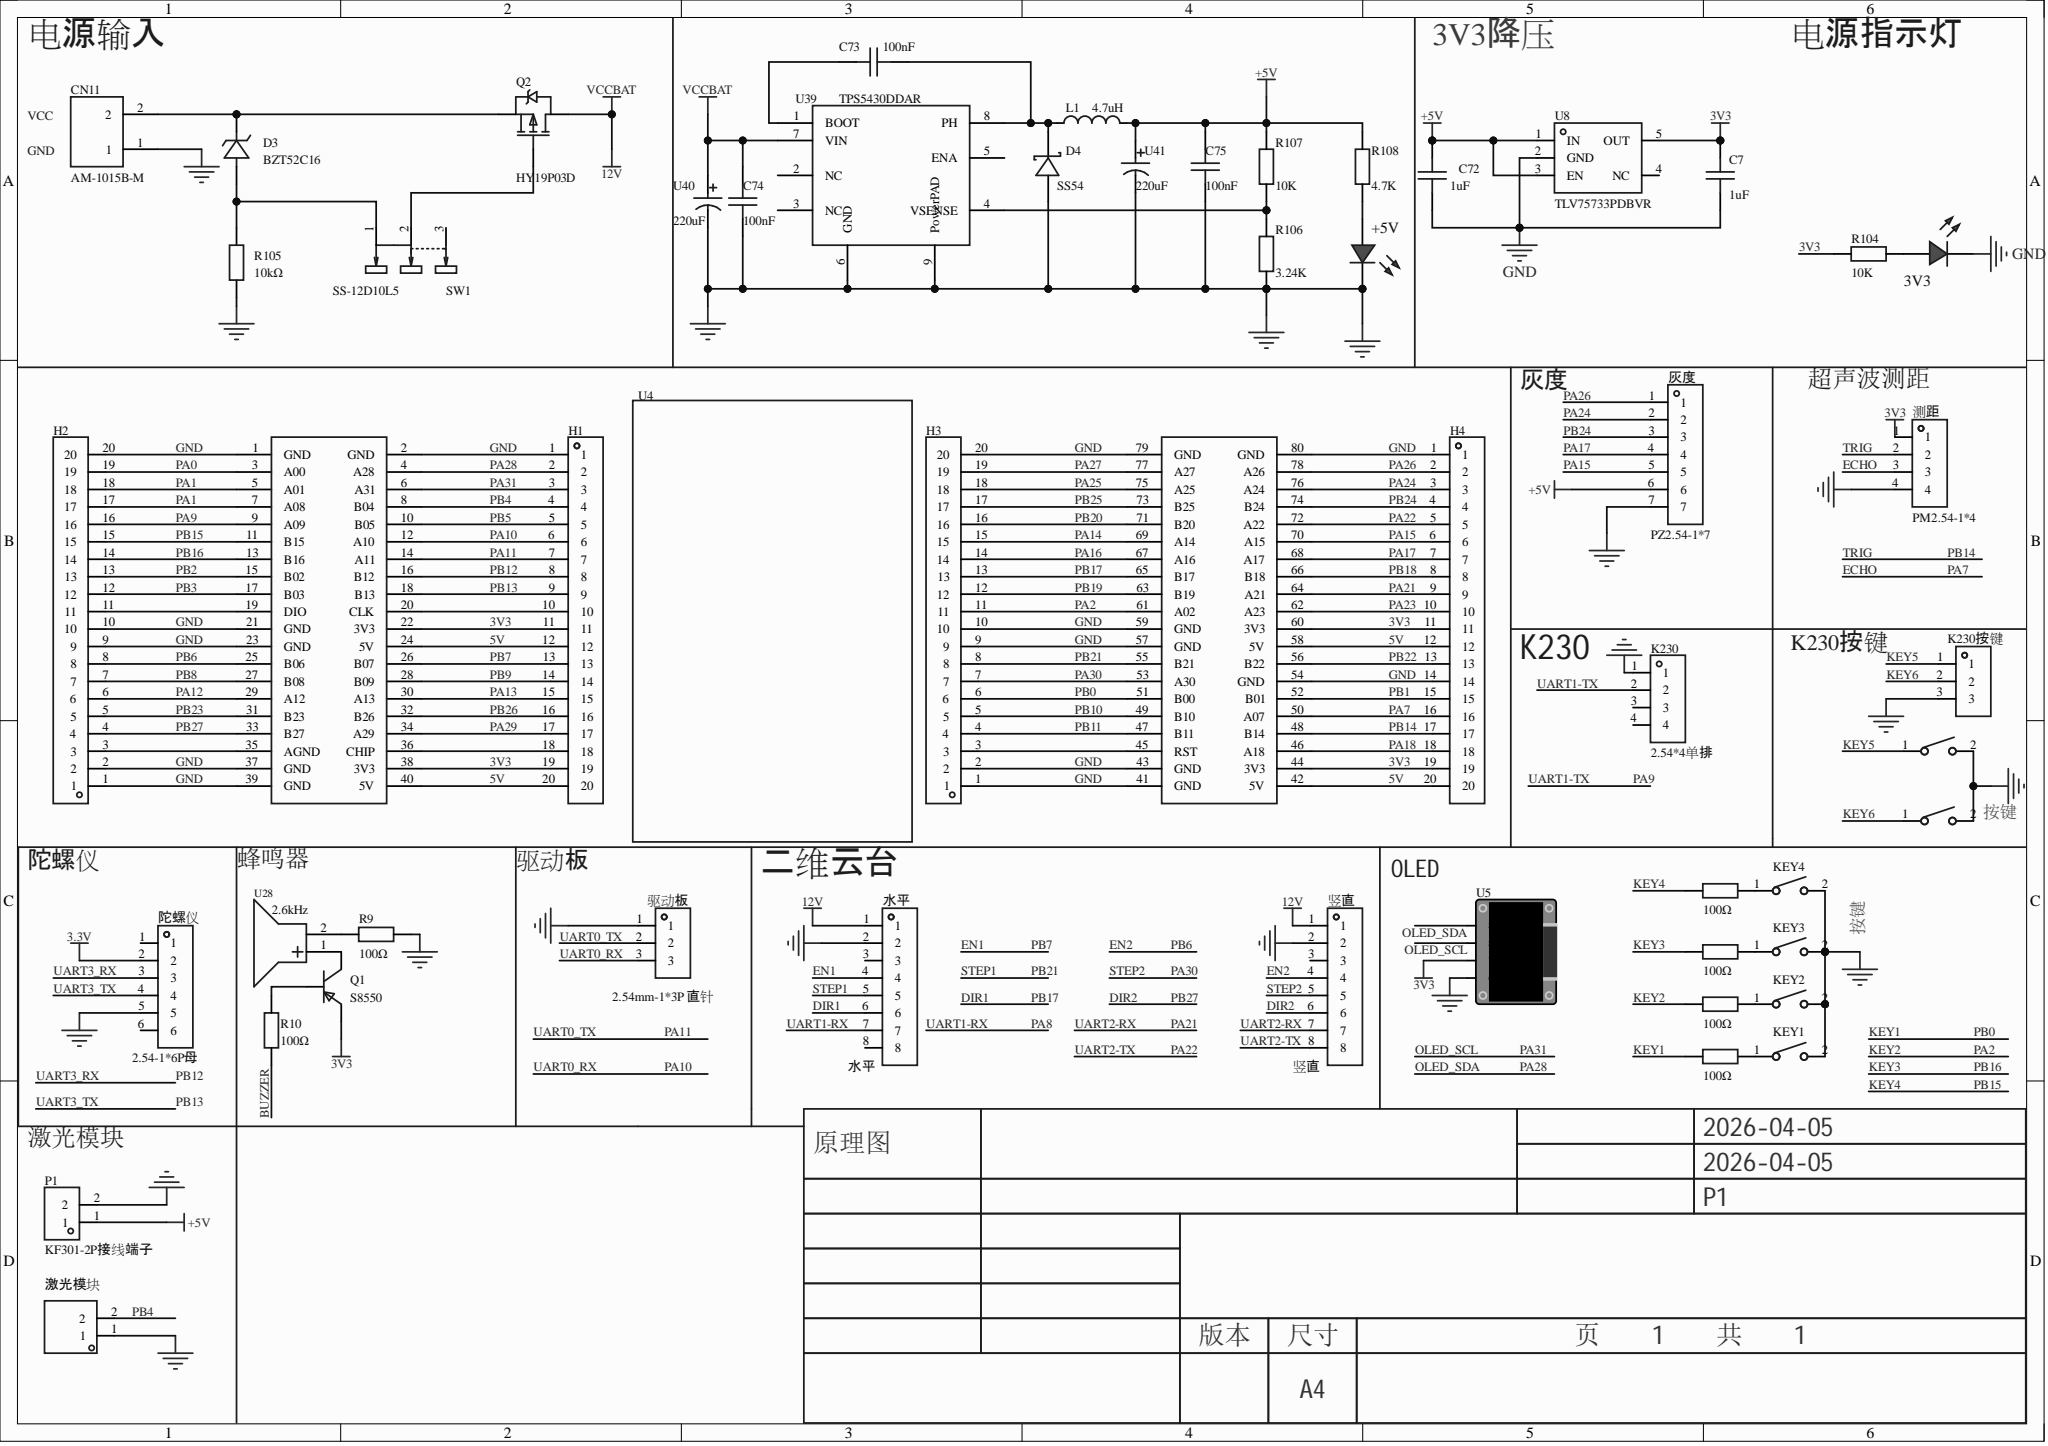Circuit board | Altium Designer | 52 parts | 80 nets
Bill of materials:
Comment,Description,Designator,Footprint,LibRef,Quantity
"","","+5V, 3V3","LED_0603","LED_0603-R","2"
"1uF","","C7, C72","C0603","CAP_0603","2"
"100nF","容值:100nF;精度:±10%;额定电压:50V;温度系数:X7R;","C73, C74, C75","C0805","CC0805KRX7R9BB104","3"
"AM-1015B-M","金属材质：铜镀金  绝缘材质：PA","CN11","CONN-TH_AM-1015B-M","AM-1015B-M","1"
"BZT52C16","二极管配置:独立式;稳压值(标称值):16V;稳压值(范围):15.3V~17.1V;耗散功率(Pd):500mW;","D3","SOD-123_L2.7-W1.6-LS3.7-RD","BZT52C16","1"
"SS54","二极管配置:独立式;正向压降(Vf):550mV@5A;直流反向耐压(Vr):40V;整流电流:5A;","D4","SMA_L4.4-W2.8-LS5.4-R-RD","SS54_C22452","1"
"","间距:2.54mm;总PIN位数:20;排数:1;插针结构:-;行距:-;安装类型:直插;圆针/方针:-;额定电流:-;额定电压:-;配合针长度:-;塑高:-;触头材质:黄铜;触头镀层:-;颜色:黑色;","H1, H2, H3, H4","HDR-TH_20P-P2.54-V-M-1","HDR-M_2.54_1x20P","4"
"2.54*4单排","","K230","HDR-TH_4P-P2.54-V-M-1","2.54*4单排","1"
"K230按键","","K230按键","HDR-TH_3P-P2.54-V-M","HDR-M_2.54_1x3P","1"
"轻触按键3*6*2.5","","K230按键1, K230按键2, KEY1, KEY2, KEY3, KEY4","SW-SMD_L6.0-W3.6-LS8.0","轻触按键3*6*2.5","6"
"4.7uH","电感值:4.7uH;精度:±20%;额定电流:5.5A;饱和电流(Isat):7A;","L1","IND-SMD_L7.3-W6.6","MCS0630-4R7MPY1","1"
"KF301-2P接线端子","","P1","CONN-TH_XY301V-A-5.0-2P","KF301-2P接线端子","1"
"S8550","晶体管类型:PNP;集电极电流(Ic):500mA;集射极击穿电压(Vceo):25V;功率(Pd):300mW;直流电流增益(hFE@Ic,Vce):120@50mA,1V;","Q1","SOT-23-3_L2.9-W1.6-P1.90-LS2.8-BR","S8550_C105432","1"
"HY19P03D","","Q2","TO-252-2_L6.6-W6.1-P4.57-LS9.9-TL-CW","HY19P03D","1"
"100Ω","","R9, R10, R109, R110, R111, R112","R0603","Res_0603, 0603WAF1000T5E","6"
"10K","","R104, R107","R0603","Res_0603","2"
"10kΩ","","R105","R0603","0603WAF1002T5E","1"
"3.24K","","R106","R0603","Res_0603","1"
"4.7K","","R108","R0603","Res_0603","1"
"SS-12D10L5","电路结构:单刀双掷;安装方式:直插;开关颜色:黑色;额定电流(DC):3A;额定电压(DC):125V;额定电流(AC):3A;额定电压(AC):125V;机械寿命:1万次;","SW1","SW-TH_SS-12D10L5","SS-12D10L5","1"
"","","U4","COMM-TH_LCKFB-TMX-MSPM0G3507","LCKFB-TMX-MSPM0G3507","1"
"","","U5","0.96OLED_4P","0.96OLED模块_4P","1"
"TLV75733PDBVR","输出类型:固定;最大输入电压:5.5V;输出电压:3.3V;输出电流:1A;电源纹波抑制比(PSRR):52dB;输出极性:正极;","U8","SOT-23-5_L2.9-W1.6-P0.95-LS2.8-BL","TLV75733PDBVR","1"
"2.6kHz","频率:2.6kHz;声压(SPL):80dB@5V,10cm;","U28","BUZ-TH_BD12.0-P7.60-D0.6-FD","HYE1206-05ST","1"
"TPS5430DDAR","功能类型:降压型;输出类型:可调;输入电压:5.5V~36V;输出电压:1.221V~32.04V;输出电流(最大值):3A;","U39","ESOP-8_L4.9-W3.9-P1.27-LS6.0-TL-EP","TPS5430DDAR","1"
"220uF","","U40, U41","CAP-SMD_BD6.3-L6.6-W6.6-LS7.2-FD","220uF","2"
"","","","CONN-TH_8P-P2.50-XH2.54-8P","XH2.54-8P 直插","1"
"PM2.54-1*4","插孔结构:1x4P;间距:2.54mm;行距:2.54mm;圆孔/方孔:方孔;安装方式:直插;排数:单排;总孔位数:4P;额定电流:2.5A;插孔方向:顶部;塑高:8.5mm;工作温度:-40℃~+105℃;","测距","HDR-TH_4P-P2.54-V-F","PM2.54-1*4","1"
"","","激光模块","HDR-TH_2P-P2.54-V-M-1","HDR-M_2.54_1x2P","1"
"PZ2.54-1*7","插针结构:1x7P;间距:2.54mm;圆针/方针:方针;安装方式:直插;排数:单排;总PIN位数:7P;额定电流:2.5A;配合针长度:6mm;塑高:2.54mm;端接针长度:3mm;触头材质:黄铜;触头镀层:金;工作温度:-40℃~+105℃;","灰度","HDR-TH_7P-P2.54-V-M","PZ2.54-1*7","1"
"","","","CONN-TH_8P-P2.50-XH2.54-8P","XH2.54-8P 直插","1"
"2.54-1*6P母","插孔结构:1x6P;间距:2.54mm;行距:-;圆孔/方孔:方孔;安装方式:直插;排数:单排;总孔位数:6P;额定电流:3A;额定电压:-;插孔方向:顶部;塑高:-;触头材质:黄铜;触头镀层:-;工作温度:-40℃~+105℃;","陀螺仪","HDR-TH_6P-P2.54-V-F","2.54-1*6P母","1"
"2.54mm-1*3P 直针","","驱动板","HDR-TH_3P-P2.54-V-M-1","2.54mm-1*3P 直针","1"
Netlist (Protel format):
[
3V3
LED_0603




]
[
+5V
LED_0603




]
[
C7
C0603
1uF



]
[
C72
C0603
1uF



]
[
C73
C0805
100nF



]
[
C74
C0805
100nF



]
[
C75
C0805
100nF



]
[
CN11
CONN-TH_AM-1015B-M
AM-1015B-M



]
[
D3
SOD-123_L2.7-W1.6-LS3.7-RD
BZT52C16



]
[
D4
SMA_L4.4-W2.8-LS5.4-R-RD
SS54



]
[
H1
HDR-TH_20P-P2.54-V-M-1




]
[
H2
HDR-TH_20P-P2.54-V-M-1




]
[
H3
HDR-TH_20P-P2.54-V-M-1




]
[
H4
HDR-TH_20P-P2.54-V-M-1




]
[
K230
HDR-TH_4P-P2.54-V-M-1
2.54*4单排



]
[
K230按键
HDR-TH_3P-P2.54-V-M
K230按键



]
[
K230按键1
SW-SMD_L6.0-W3.6-LS8.0
轻触按键3*6*2.5



]
[
K230按键2
SW-SMD_L6.0-W3.6-LS8.0
轻触按键3*6*2.5



]
[
KEY1
SW-SMD_L6.0-W3.6-LS8.0
轻触按键3*6*2.5



]
[
KEY2
SW-SMD_L6.0-W3.6-LS8.0
轻触按键3*6*2.5



]
[
KEY3
SW-SMD_L6.0-W3.6-LS8.0
轻触按键3*6*2.5



]
[
KEY4
SW-SMD_L6.0-W3.6-LS8.0
轻触按键3*6*2.5



]
[
L1
IND-SMD_L7.3-W6.6
4.7uH



]
[
P1
CONN-TH_XY301V-A-5.0-2P
KF301-2P接线端子



]
[
Q1
SOT-23-3_L2.9-W1.6-P1.90-LS2.8-BR
S8550



]
[
Q2
TO-252-2_L6.6-W6.1-P4.57-LS9.9-TL-CW
HY19P03D



]
[
R9
R0603
100Ω



]
[
R10
R0603
100Ω



]
[
R104
R0603
10K



]
[
R105
R0603
10kΩ



]
[
R106
R0603
3.24K



]
[
R107
R0603
10K



]
[
R108
R0603
4.7K



]
[
R109
R0603
100Ω



]
[
R110
R0603
100Ω



]
[
R111
R0603
100Ω



]
[
R112
R0603
100Ω



]
[
SW1
SW-TH_SS-12D10L5
SS-12D10L5



]
[
U4
COMM-TH_LCKFB-TMX-MSPM0G3507




]
[
U5
0.96OLED_4P




]
[
U8
SOT-23-5_L2.9-W1.6-P0.95-LS2.8-BL
TLV75733PDBVR



]
[
U28
BUZ-TH_BD12.0-P7.60-D0.6-FD
2.6kHz



]
[
U39
ESOP-8_L4.9-W3.9-P1.27-LS6.0-TL-EP
TPS5430DDAR



]
[
U40
CAP-SMD_BD6.3-L6.6-W6.6-LS7.2-FD
220uF



]
[
U41
CAP-SMD_BD6.3-L6.6-W6.6-LS7.2-FD
220uF



]
[
水平
CONN-TH_8P-P2.50-XH2.54-8P
水平



]
[
测距
HDR-TH_4P-P2.54-V-F
PM2.54-1*4



]
[
激光模块
HDR-TH_2P-P2.54-V-M-1




]
[
灰度
HDR-TH_7P-P2.54-V-M
PZ2.54-1*7



]
[
竖直
CONN-TH_8P-P2.50-XH2.54-8P
竖直



]
[
陀螺仪
HDR-TH_6P-P2.54-V-F
2.54-1*6P母



]
[
驱动板
HDR-TH_3P-P2.54-V-M-1
2.54mm-1*3P 直针



]
(
PB26
H1-16
U4-32
)
(
PB25
H3-17
U4-73
)
(
PB24
H4-4
U4-74
灰度-3
)
(
PB23
H2-5
U4-31
)
(
PB22
H4-13
U4-56
)
(
PB21
H3-8
U4-55
水平-5
)
(
PB20
H3-16
U4-71
)
(
PB19
H3-12
U4-63
)
(
PB18
H4-8
U4-66
)
(
PB14
H4-17
U4-48
测距-2
)
(
PB13
H1-9
U4-18
陀螺仪-4
)
(
PB12
H1-8
U4-16
陀螺仪-3
)
(
PB11
H3-4
U4-47
)
(
PB10
H3-5
U4-49
)
(
PB9
H1-14
U4-28
)
(
PB8
H2-7
U4-27
)
(
PB5
H1-5
U4-10
)
(
PB4
H1-4
U4-8
激光模块-2
)
(
PB3
H2-12
U4-17
)
(
PB2
H2-13
U4-15
)
(
PB1
H4-15
U4-52
)
(
PA30
H3-7
U4-53
竖直-5
)
(
PA29
H1-17
U4-34
)
(
PA27
H3-19
U4-77
)
(
PA26
H4-2
U4-78
灰度-1
)
(
PA25
H3-18
U4-75
)
(
PA24
H4-3
U4-76
灰度-2
)
(
PA23
H4-10
U4-62
)
(
PA22
H4-5
U4-72
竖直-8
)
(
PA21
H4-9
U4-64
竖直-7
)
(
PA18
H4-18
U4-46
)
(
PA17
H4-7
U4-68
灰度-4
)
(
PA16
H3-14
U4-67
)
(
PA15
H4-6
U4-70
灰度-5
)
(
PA14
H3-15
U4-69
)
(
PA13
H1-15
U4-30
)
(
PA12
H2-6
U4-29
)
(
PA11
H1-7
U4-14
驱动板-2
)
(
PA10
H1-6
U4-12
驱动板-3
)
(
PA9
H2-16
K230-2
U4-9
)
(
PA1
H2-17
H2-18
U4-5
U4-7
)
(
PA0
H2-19
U4-3
)
(
OLED_SDA
H1-2
U4-4
U5-4
)
(
OLED_SCL
H1-3
U4-6
U5-3
)
(
NetR106_2
R106-2
R107-1
U39-4
)
(
NetR9_2
R9-2
U28-2
)
(
NetQ2_1
Q2-1
SW1-2
)
(
NetQ1_3
Q1-3
U28-1
)
(
NetQ1_1
Q1-1
R10-1
)
(
NetKEY4_1
KEY4-1
R112-1
)
(
NetKEY3_1
KEY3-1
R111-1
)
(
NetKEY2_1
KEY2-1
R110-1
)
(
NetKEY1_1
KEY1-1
R109-1
)
(
NetH3_3
H3-3
U4-45
)
(
NetH2_11
H2-11
U4-19
)
(
NetH2_3
H2-3
U4-35
)
(
NetH1_18
H1-18
U4-36
)
(
NetH1_10
H1-10
U4-20
)
(
NetD3_2
D3-2
R105-2
SW1-1
)
(
NetCN11_2
CN11-2
D3-1
Q2-3
)
(
NetC73_2
C73-2
D4-2
L1-1
U39-8
)
(
NetC73_1
C73-1
U39-1
)
(
Net+5V_2
+5V-2
R108-1
)
(
Net3V3_2
3V3-2
R104-2
)
(
KEY6
K230按键-2
K230按键2-1
)
(
KEY5
K230按键-1
K230按键1-1
)
(
KEY4
H2-15
R112-2
U4-11
)
(
KEY3
H2-14
R111-2
U4-13
)
(
KEY2
H3-11
R110-2
U4-61
)
(
KEY1
H3-6
R109-2
U4-51
)
(
GND
3V3-1
+5V-1
C7-1
C72-1
C74-1
C75-1
CN11-1
D4-1
H1-1
H2-1
H2-2
H2-9
H2-10
H2-20
H3-1
H3-2
H3-9
H3-10
H3-20
H4-1
H4-14
K230-1
K230按键-3
K230按键1-2
K230按键2-2
KEY1-2
KEY2-2
KEY3-2
KEY4-2
P1-2
R9-1
R105-1
R106-1
U4-1
U4-2
U4-21
U4-23
U4-37
U4-39
U4-41
U4-43
U4-54
U4-57
U4-59
U4-79
U4-80
U5-1
U8-2
U39-6
U39-9
U40-2
U41-2
水平-2
测距-4
激光模块-1
灰度-7
竖直-2
陀螺仪-5
驱动板-1
)
(
EN2
H2-8
U4-25
竖直-4
)
(
EN1
H1-13
U4-26
水平-4
)
(
ECHO
H4-16
U4-50
测距-3
)
(
DIR2
H2-4
U4-33
竖直-6
)
(
DIR1
H3-13
U4-65
水平-6
)
(
+5V
C72-2
C75-2
L1-2
P1-1
R107-2
R108-2
U8-1
U8-3
U41-1
灰度-6
)
(
12V
C74-2
Q2-2
U39-7
U40-1
水平-1
竖直-1
)
(
5V
H1-12
H1-20
H4-12
H4-20
U4-24
U4-40
U4-42
U4-58
)
(
3V3
C7-2
H1-11
H1-19
H4-11
H4-19
Q1-2
R104-1
U4-22
U4-38
U4-44
U4-60
U5-2
U8-5
测距-1
)